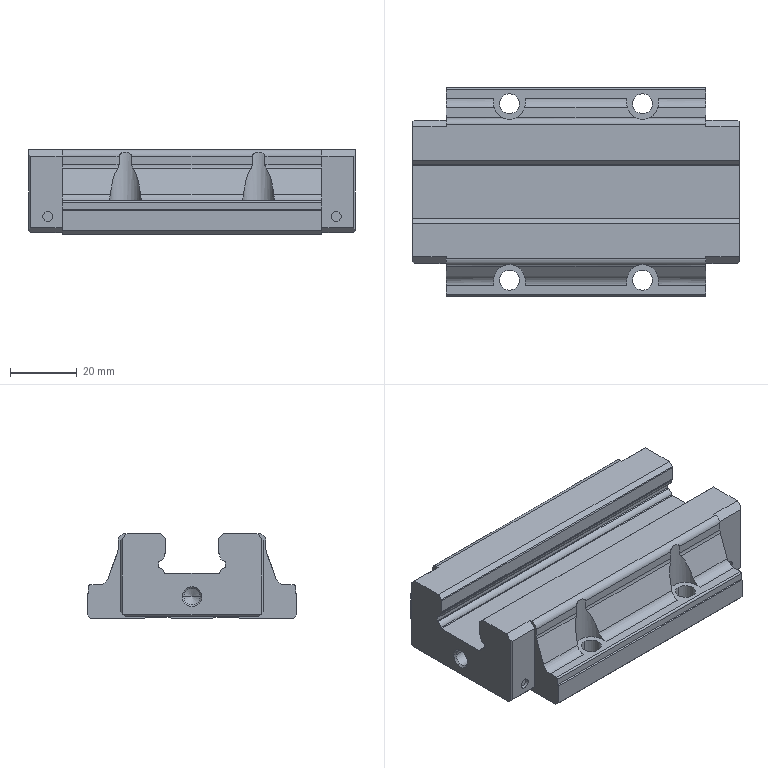Part | STEP file | [SHS20LC1SS僽儘僢僋]-4 | 1 solid | 146 faces | box 98 x 63 x 25.4 mm | volume 103965 mm3 | plane 76 | cylinder 62 | cone 8 | commonest cylinder face diameters 6 x20 0.4 x9 3 x8 1 x6 9.5 x6 3.604 x5